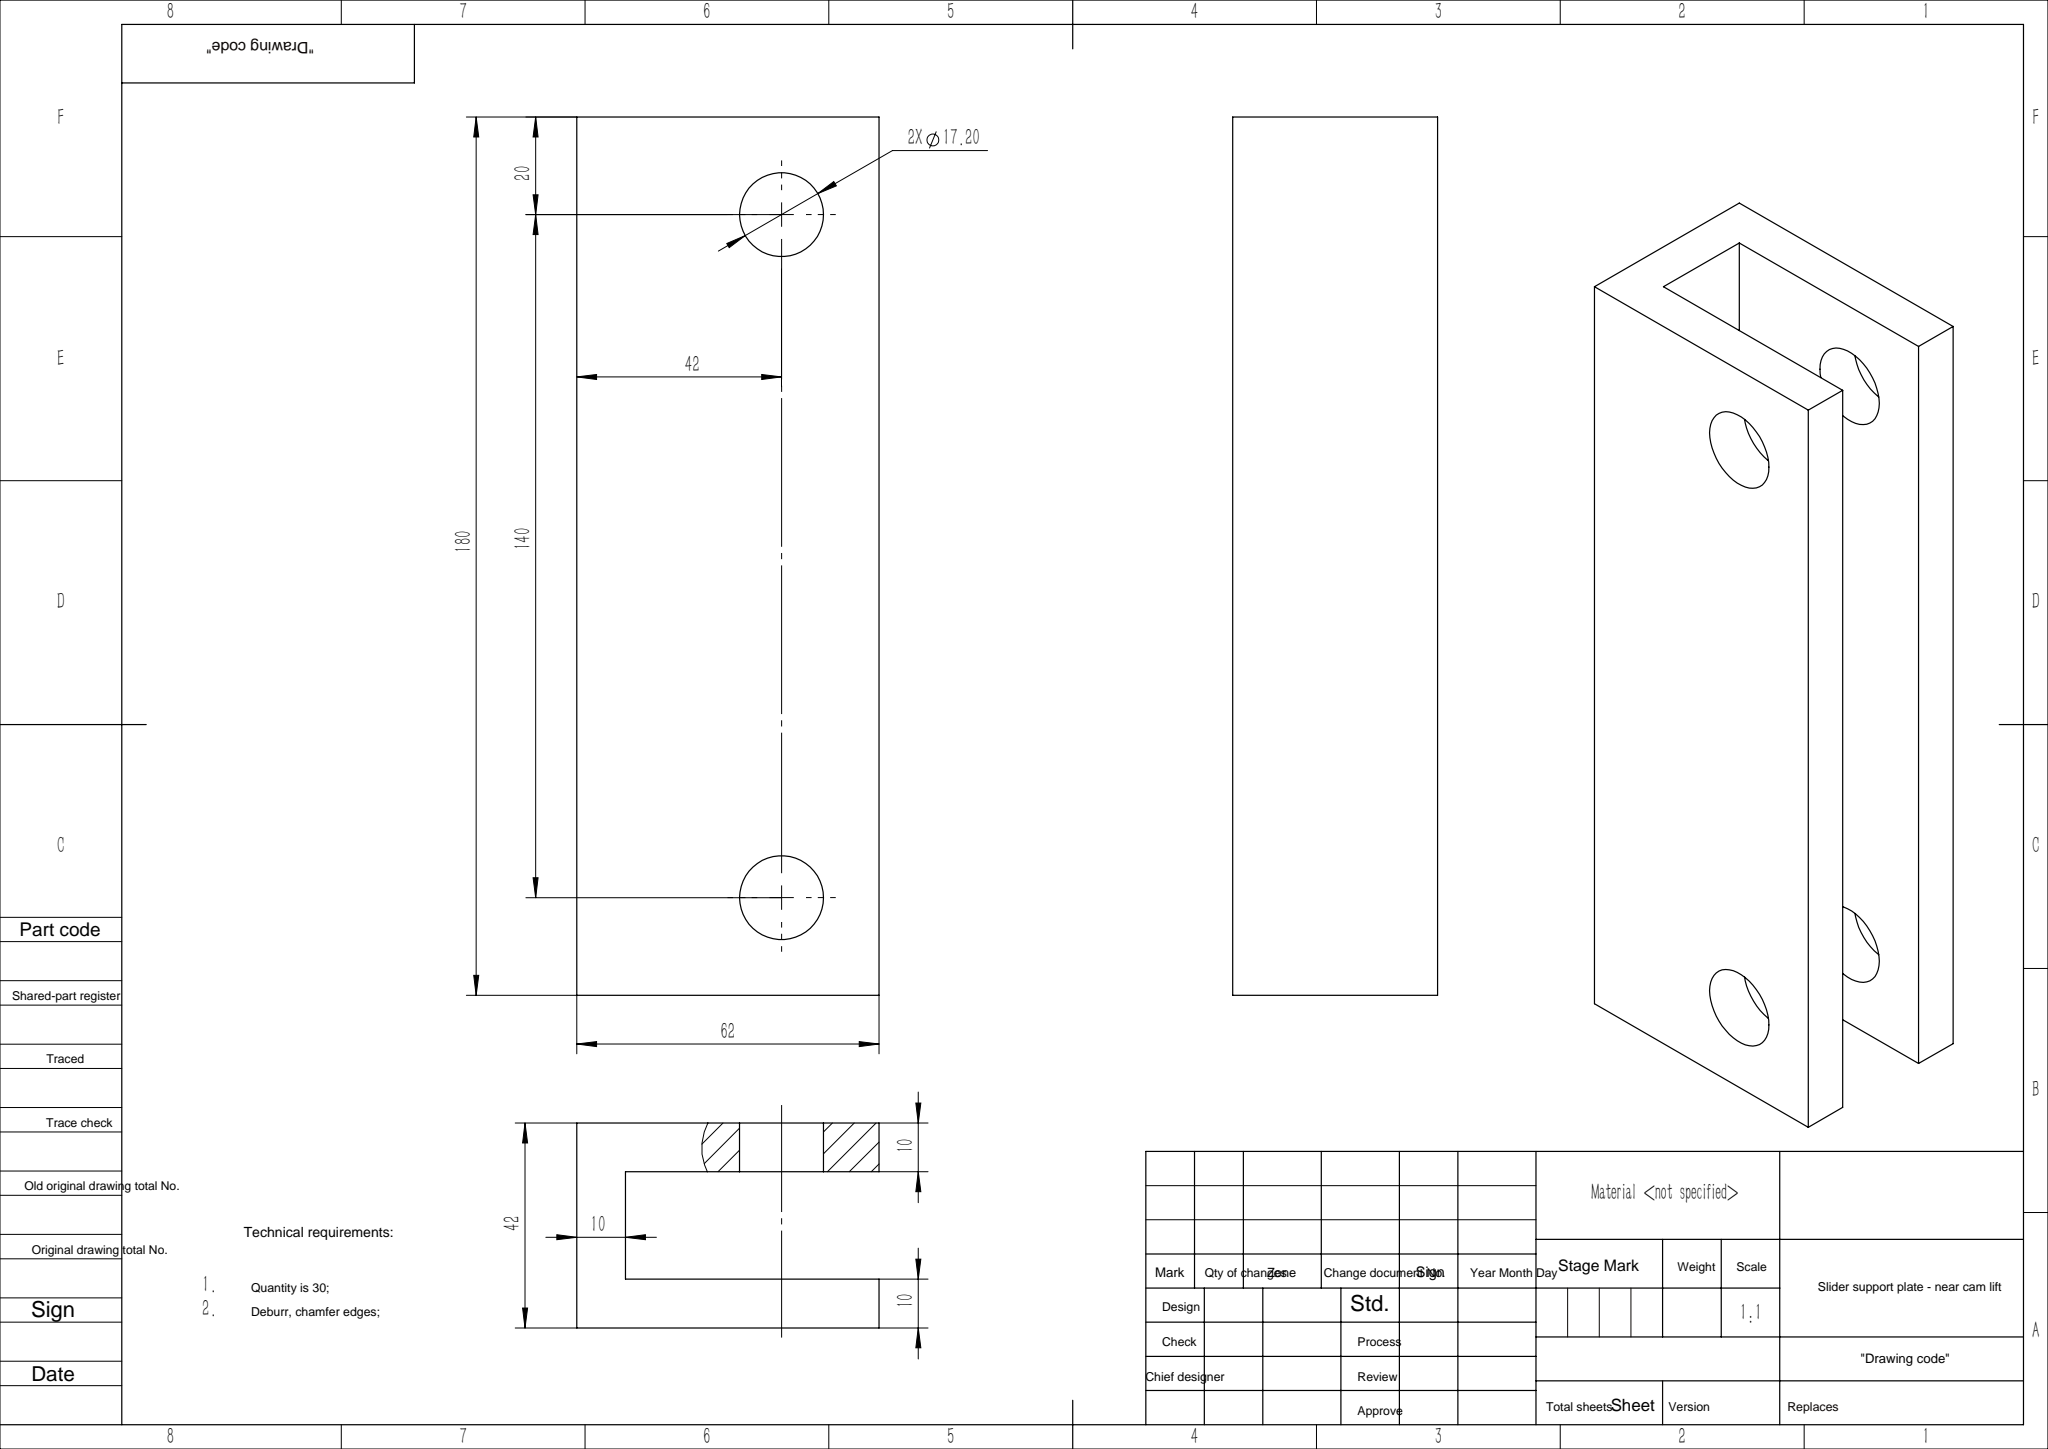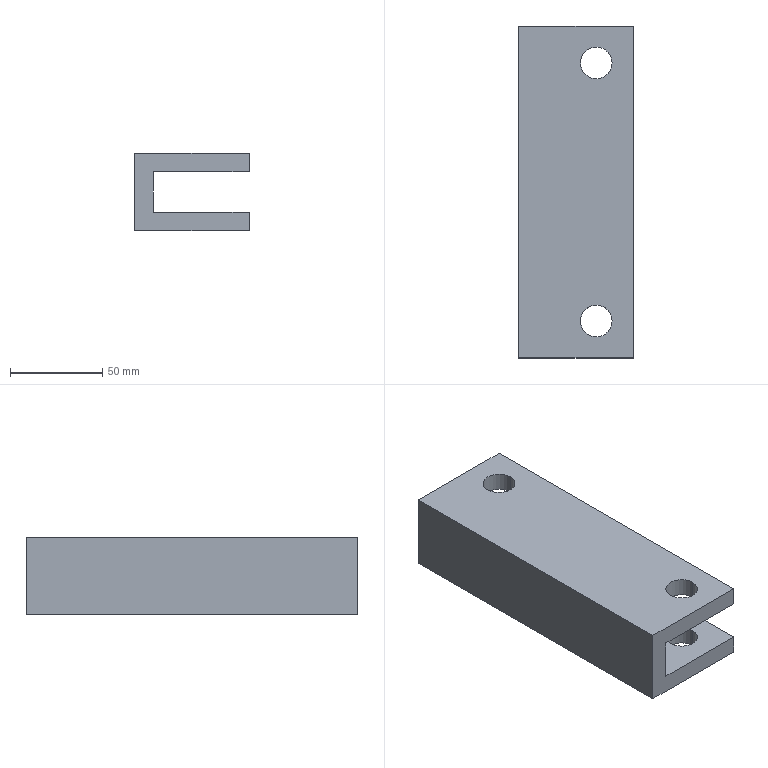Part | SolidWorks | features Extrusion 1, ICE 1 | 1 solid | 18 faces | box 62 x 180 x 42 mm | volume 253506 mm3 | plane 10 | cylinder 8 | commonest cylinder face diameters 17.2 x8
STEP:
#1=CARTESIAN_POINT('',(33.4,20.,11.));
#2=VERTEX_POINT('',#1);
#3=CARTESIAN_POINT('',(50.6,20.,11.));
#4=VERTEX_POINT('',#3);
#5=CARTESIAN_POINT('',(42.,20.,11.));
#6=DIRECTION('',(0.,0.,1.));
#7=DIRECTION('',(1.,0.,0.));
#8=AXIS2_PLACEMENT_3D('',#5,#6,#7);
#9=CIRCLE('',#8,8.6);
#10=EDGE_CURVE('',#2,#4,#9,.T.);
#11=ORIENTED_EDGE('',*,*,#10,.F.);
#12=CARTESIAN_POINT('',(33.4,20.,21.));
#13=VERTEX_POINT('',#12);
#14=CARTESIAN_POINT('',(33.4,20.,-21.));
#15=DIRECTION('',(0.,0.,1.));
#16=VECTOR('',#15,1000.);
#17=LINE('',#14,#16);
#18=EDGE_CURVE('',#2,#13,#17,.T.);
#19=ORIENTED_EDGE('',*,*,#18,.T.);
#20=CARTESIAN_POINT('',(50.6,20.,21.));
#21=VERTEX_POINT('',#20);
#22=CARTESIAN_POINT('',(42.,20.,21.));
#23=DIRECTION('',(0.,0.,1.));
#24=DIRECTION('',(1.,0.,0.));
#25=AXIS2_PLACEMENT_3D('',#22,#23,#24);
#26=CIRCLE('',#25,8.6);
#27=EDGE_CURVE('',#13,#21,#26,.T.);
#28=ORIENTED_EDGE('',*,*,#27,.T.);
#29=CARTESIAN_POINT('',(50.6,20.,-21.));
#30=DIRECTION('',(0.,0.,1.));
#31=VECTOR('',#30,1000.);
#32=LINE('',#29,#31);
#33=EDGE_CURVE('',#4,#21,#32,.T.);
#34=ORIENTED_EDGE('',*,*,#33,.F.);
#35=EDGE_LOOP('',(#11,#19,#28,#34));
#36=FACE_OUTER_BOUND('',#35,.T.);
#37=CARTESIAN_POINT('',(42.,20.,-21.));
#38=DIRECTION('',(0.,0.,1.));
#39=DIRECTION('',(1.,0.,0.));
#40=AXIS2_PLACEMENT_3D('',#37,#38,#39);
#41=CYLINDRICAL_SURFACE('',#40,8.6);
#42=ADVANCED_FACE('',(#36),#41,.F.);
#43=CARTESIAN_POINT('',(33.4,20.,-21.));
#44=VERTEX_POINT('',#43);
#45=CARTESIAN_POINT('',(50.6,20.,-21.));
#46=VERTEX_POINT('',#45);
#47=CARTESIAN_POINT('',(42.,20.,-21.));
#48=DIRECTION('',(0.,0.,1.));
#49=DIRECTION('',(1.,0.,0.));
#50=AXIS2_PLACEMENT_3D('',#47,#48,#49);
#51=CIRCLE('',#50,8.6);
#52=EDGE_CURVE('',#44,#46,#51,.T.);
#53=ORIENTED_EDGE('',*,*,#52,.F.);
#54=CARTESIAN_POINT('',(33.4,20.,-11.));
#55=VERTEX_POINT('',#54);
#56=CARTESIAN_POINT('',(33.4,20.,-21.));
#57=DIRECTION('',(0.,0.,1.));
#58=VECTOR('',#57,1000.);
#59=LINE('',#56,#58);
#60=EDGE_CURVE('',#44,#55,#59,.T.);
#61=ORIENTED_EDGE('',*,*,#60,.T.);
#62=CARTESIAN_POINT('',(50.6,20.,-11.));
#63=VERTEX_POINT('',#62);
#64=CARTESIAN_POINT('',(42.,20.,-11.));
#65=DIRECTION('',(0.,0.,-1.));
#66=DIRECTION('',(-1.,0.,0.));
#67=AXIS2_PLACEMENT_3D('',#64,#65,#66);
#68=CIRCLE('',#67,8.6);
#69=EDGE_CURVE('',#63,#55,#68,.T.);
#70=ORIENTED_EDGE('',*,*,#69,.F.);
#71=CARTESIAN_POINT('',(50.6,20.,-21.));
#72=DIRECTION('',(0.,0.,1.));
#73=VECTOR('',#72,1000.);
#74=LINE('',#71,#73);
#75=EDGE_CURVE('',#46,#63,#74,.T.);
#76=ORIENTED_EDGE('',*,*,#75,.F.);
#77=EDGE_LOOP('',(#53,#61,#70,#76));
#78=FACE_OUTER_BOUND('',#77,.T.);
#79=CARTESIAN_POINT('',(42.,20.,-21.));
#80=DIRECTION('',(0.,0.,1.));
#81=DIRECTION('',(1.,0.,0.));
#82=AXIS2_PLACEMENT_3D('',#79,#80,#81);
#83=CYLINDRICAL_SURFACE('',#82,8.6);
#84=ADVANCED_FACE('',(#78),#83,.F.);
#85=CARTESIAN_POINT('',(33.4,160.,11.));
#86=VERTEX_POINT('',#85);
#87=CARTESIAN_POINT('',(50.6,160.,11.));
#88=VERTEX_POINT('',#87);
#89=CARTESIAN_POINT('',(42.,160.,11.));
#90=DIRECTION('',(0.,0.,1.));
#91=DIRECTION('',(1.,0.,0.));
#92=AXIS2_PLACEMENT_3D('',#89,#90,#91);
#93=CIRCLE('',#92,8.6);
#94=EDGE_CURVE('',#86,#88,#93,.T.);
#95=ORIENTED_EDGE('',*,*,#94,.F.);
#96=CARTESIAN_POINT('',(33.4,160.,21.));
#97=VERTEX_POINT('',#96);
#98=CARTESIAN_POINT('',(33.4,160.,-21.));
#99=DIRECTION('',(0.,0.,1.));
#100=VECTOR('',#99,1000.);
#101=LINE('',#98,#100);
#102=EDGE_CURVE('',#86,#97,#101,.T.);
#103=ORIENTED_EDGE('',*,*,#102,.T.);
#104=CARTESIAN_POINT('',(50.6,160.,21.));
#105=VERTEX_POINT('',#104);
#106=CARTESIAN_POINT('',(42.,160.,21.));
#107=DIRECTION('',(0.,0.,1.));
#108=DIRECTION('',(1.,0.,0.));
#109=AXIS2_PLACEMENT_3D('',#106,#107,#108);
#110=CIRCLE('',#109,8.6);
#111=EDGE_CURVE('',#97,#105,#110,.T.);
#112=ORIENTED_EDGE('',*,*,#111,.T.);
#113=CARTESIAN_POINT('',(50.6,160.,-21.));
#114=DIRECTION('',(0.,0.,1.));
#115=VECTOR('',#114,1000.);
#116=LINE('',#113,#115);
#117=EDGE_CURVE('',#88,#105,#116,.T.);
#118=ORIENTED_EDGE('',*,*,#117,.F.);
#119=EDGE_LOOP('',(#95,#103,#112,#118));
#120=FACE_OUTER_BOUND('',#119,.T.);
#121=CARTESIAN_POINT('',(42.,160.,-21.));
#122=DIRECTION('',(0.,0.,1.));
#123=DIRECTION('',(1.,0.,0.));
#124=AXIS2_PLACEMENT_3D('',#121,#122,#123);
#125=CYLINDRICAL_SURFACE('',#124,8.6);
#126=ADVANCED_FACE('',(#120),#125,.F.);
#127=CARTESIAN_POINT('',(33.4,160.,-21.));
#128=VERTEX_POINT('',#127);
#129=CARTESIAN_POINT('',(50.6,160.,-21.));
#130=VERTEX_POINT('',#129);
#131=CARTESIAN_POINT('',(42.,160.,-21.));
#132=DIRECTION('',(0.,0.,1.));
#133=DIRECTION('',(1.,0.,0.));
#134=AXIS2_PLACEMENT_3D('',#131,#132,#133);
#135=CIRCLE('',#134,8.6);
#136=EDGE_CURVE('',#128,#130,#135,.T.);
#137=ORIENTED_EDGE('',*,*,#136,.F.);
#138=CARTESIAN_POINT('',(33.4,160.,-11.));
#139=VERTEX_POINT('',#138);
#140=CARTESIAN_POINT('',(33.4,160.,-21.));
#141=DIRECTION('',(0.,0.,1.));
#142=VECTOR('',#141,1000.);
#143=LINE('',#140,#142);
#144=EDGE_CURVE('',#128,#139,#143,.T.);
#145=ORIENTED_EDGE('',*,*,#144,.T.);
#146=CARTESIAN_POINT('',(50.6,160.,-11.));
#147=VERTEX_POINT('',#146);
#148=CARTESIAN_POINT('',(42.,160.,-11.));
#149=DIRECTION('',(0.,0.,-1.));
#150=DIRECTION('',(-1.,0.,0.));
#151=AXIS2_PLACEMENT_3D('',#148,#149,#150);
#152=CIRCLE('',#151,8.6);
#153=EDGE_CURVE('',#147,#139,#152,.T.);
#154=ORIENTED_EDGE('',*,*,#153,.F.);
#155=CARTESIAN_POINT('',(50.6,160.,-21.));
#156=DIRECTION('',(0.,0.,1.));
#157=VECTOR('',#156,1000.);
#158=LINE('',#155,#157);
#159=EDGE_CURVE('',#130,#147,#158,.T.);
#160=ORIENTED_EDGE('',*,*,#159,.F.);
#161=EDGE_LOOP('',(#137,#145,#154,#160));
#162=FACE_OUTER_BOUND('',#161,.T.);
#163=CARTESIAN_POINT('',(42.,160.,-21.));
#164=DIRECTION('',(0.,0.,1.));
#165=DIRECTION('',(1.,0.,0.));
#166=AXIS2_PLACEMENT_3D('',#163,#164,#165);
#167=CYLINDRICAL_SURFACE('',#166,8.6);
#168=ADVANCED_FACE('',(#162),#167,.F.);
#169=CARTESIAN_POINT('',(0.,0.,-21.));
#170=VERTEX_POINT('',#169);
#171=CARTESIAN_POINT('',(0.,0.,21.));
#172=VERTEX_POINT('',#171);
#173=CARTESIAN_POINT('',(0.,0.,-21.));
#174=DIRECTION('',(0.,0.,1.));
#175=VECTOR('',#174,1000.);
#176=LINE('',#173,#175);
#177=EDGE_CURVE('',#170,#172,#176,.T.);
#178=ORIENTED_EDGE('',*,*,#177,.T.);
#179=CARTESIAN_POINT('',(0.,180.,21.));
#180=VERTEX_POINT('',#179);
#181=CARTESIAN_POINT('',(0.,180.,21.));
#182=DIRECTION('',(0.,-1.,0.));
#183=VECTOR('',#182,1000.);
#184=LINE('',#181,#183);
#185=EDGE_CURVE('',#180,#172,#184,.T.);
#186=ORIENTED_EDGE('',*,*,#185,.F.);
#187=CARTESIAN_POINT('',(0.,180.,-21.));
#188=VERTEX_POINT('',#187);
#189=CARTESIAN_POINT('',(0.,180.,-21.));
#190=DIRECTION('',(0.,0.,1.));
#191=VECTOR('',#190,1000.);
#192=LINE('',#189,#191);
#193=EDGE_CURVE('',#188,#180,#192,.T.);
#194=ORIENTED_EDGE('',*,*,#193,.F.);
#195=CARTESIAN_POINT('',(0.,180.,-21.));
#196=DIRECTION('',(0.,-1.,0.));
#197=VECTOR('',#196,1000.);
#198=LINE('',#195,#197);
#199=EDGE_CURVE('',#188,#170,#198,.T.);
#200=ORIENTED_EDGE('',*,*,#199,.T.);
#201=EDGE_LOOP('',(#178,#186,#194,#200));
#202=FACE_OUTER_BOUND('',#201,.T.);
#203=CARTESIAN_POINT('',(0.,180.,-21.));
#204=DIRECTION('',(1.,0.,0.));
#205=DIRECTION('',(0.,0.,-1.));
#206=AXIS2_PLACEMENT_3D('',#203,#204,#205);
#207=PLANE('',#206);
#208=ADVANCED_FACE('',(#202),#207,.F.);
#209=CARTESIAN_POINT('',(42.,20.,21.));
#210=DIRECTION('',(0.,0.,1.));
#211=DIRECTION('',(1.,0.,0.));
#212=AXIS2_PLACEMENT_3D('',#209,#210,#211);
#213=CIRCLE('',#212,8.6);
#214=EDGE_CURVE('',#21,#13,#213,.T.);
#215=ORIENTED_EDGE('',*,*,#214,.F.);
#216=ORIENTED_EDGE('',*,*,#27,.F.);
#217=EDGE_LOOP('',(#215,#216));
#218=FACE_BOUND('',#217,.T.);
#219=CARTESIAN_POINT('',(42.,160.,21.));
#220=DIRECTION('',(0.,0.,1.));
#221=DIRECTION('',(1.,0.,0.));
#222=AXIS2_PLACEMENT_3D('',#219,#220,#221);
#223=CIRCLE('',#222,8.6);
#224=EDGE_CURVE('',#105,#97,#223,.T.);
#225=ORIENTED_EDGE('',*,*,#224,.F.);
#226=ORIENTED_EDGE('',*,*,#111,.F.);
#227=EDGE_LOOP('',(#225,#226));
#228=FACE_BOUND('',#227,.T.);
#229=CARTESIAN_POINT('',(62.,0.,21.));
#230=VERTEX_POINT('',#229);
#231=CARTESIAN_POINT('',(0.,0.,21.));
#232=DIRECTION('',(1.,0.,0.));
#233=VECTOR('',#232,1000.);
#234=LINE('',#231,#233);
#235=EDGE_CURVE('',#172,#230,#234,.T.);
#236=ORIENTED_EDGE('',*,*,#235,.T.);
#237=CARTESIAN_POINT('',(62.,180.,21.));
#238=VERTEX_POINT('',#237);
#239=CARTESIAN_POINT('',(62.,180.,21.));
#240=DIRECTION('',(0.,-1.,0.));
#241=VECTOR('',#240,1000.);
#242=LINE('',#239,#241);
#243=EDGE_CURVE('',#238,#230,#242,.T.);
#244=ORIENTED_EDGE('',*,*,#243,.F.);
#245=CARTESIAN_POINT('',(0.,180.,21.));
#246=DIRECTION('',(1.,0.,0.));
#247=VECTOR('',#246,1000.);
#248=LINE('',#245,#247);
#249=EDGE_CURVE('',#180,#238,#248,.T.);
#250=ORIENTED_EDGE('',*,*,#249,.F.);
#251=ORIENTED_EDGE('',*,*,#185,.T.);
#252=EDGE_LOOP('',(#236,#244,#250,#251));
#253=FACE_OUTER_BOUND('',#252,.T.);
#254=CARTESIAN_POINT('',(0.,180.,21.));
#255=DIRECTION('',(0.,0.,-1.));
#256=DIRECTION('',(-1.,0.,0.));
#257=AXIS2_PLACEMENT_3D('',#254,#255,#256);
#258=PLANE('',#257);
#259=ADVANCED_FACE('',(#218,#228,#253),#258,.F.);
#260=CARTESIAN_POINT('',(62.,0.,11.));
#261=VERTEX_POINT('',#260);
#262=CARTESIAN_POINT('',(62.,0.,11.));
#263=DIRECTION('',(0.,0.,-1.));
#264=VECTOR('',#263,1000.);
#265=LINE('',#262,#264);
#266=EDGE_CURVE('',#230,#261,#265,.T.);
#267=ORIENTED_EDGE('',*,*,#266,.T.);
#268=CARTESIAN_POINT('',(62.,180.,11.));
#269=VERTEX_POINT('',#268);
#270=CARTESIAN_POINT('',(62.,180.,11.));
#271=DIRECTION('',(0.,-1.,0.));
#272=VECTOR('',#271,1000.);
#273=LINE('',#270,#272);
#274=EDGE_CURVE('',#269,#261,#273,.T.);
#275=ORIENTED_EDGE('',*,*,#274,.F.);
#276=CARTESIAN_POINT('',(62.,180.,11.));
#277=DIRECTION('',(0.,0.,-1.));
#278=VECTOR('',#277,1000.);
#279=LINE('',#276,#278);
#280=EDGE_CURVE('',#238,#269,#279,.T.);
#281=ORIENTED_EDGE('',*,*,#280,.F.);
#282=ORIENTED_EDGE('',*,*,#243,.T.);
#283=EDGE_LOOP('',(#267,#275,#281,#282));
#284=FACE_OUTER_BOUND('',#283,.T.);
#285=CARTESIAN_POINT('',(62.,180.,11.));
#286=DIRECTION('',(-1.,0.,0.));
#287=DIRECTION('',(0.,0.,1.));
#288=AXIS2_PLACEMENT_3D('',#285,#286,#287);
#289=PLANE('',#288);
#290=ADVANCED_FACE('',(#284),#289,.F.);
#291=CARTESIAN_POINT('',(42.,20.,11.));
#292=DIRECTION('',(0.,0.,1.));
#293=DIRECTION('',(1.,0.,0.));
#294=AXIS2_PLACEMENT_3D('',#291,#292,#293);
#295=CIRCLE('',#294,8.6);
#296=EDGE_CURVE('',#4,#2,#295,.T.);
#297=ORIENTED_EDGE('',*,*,#296,.T.);
#298=ORIENTED_EDGE('',*,*,#10,.T.);
#299=EDGE_LOOP('',(#297,#298));
#300=FACE_BOUND('',#299,.T.);
#301=CARTESIAN_POINT('',(42.,160.,11.));
#302=DIRECTION('',(0.,0.,1.));
#303=DIRECTION('',(1.,0.,0.));
#304=AXIS2_PLACEMENT_3D('',#301,#302,#303);
#305=CIRCLE('',#304,8.6);
#306=EDGE_CURVE('',#88,#86,#305,.T.);
#307=ORIENTED_EDGE('',*,*,#306,.T.);
#308=ORIENTED_EDGE('',*,*,#94,.T.);
#309=EDGE_LOOP('',(#307,#308));
#310=FACE_BOUND('',#309,.T.);
#311=CARTESIAN_POINT('',(10.,0.,11.));
#312=VERTEX_POINT('',#311);
#313=CARTESIAN_POINT('',(10.,0.,11.));
#314=DIRECTION('',(-1.,0.,0.));
#315=VECTOR('',#314,1000.);
#316=LINE('',#313,#315);
#317=EDGE_CURVE('',#261,#312,#316,.T.);
#318=ORIENTED_EDGE('',*,*,#317,.T.);
#319=CARTESIAN_POINT('',(10.,180.,11.));
#320=VERTEX_POINT('',#319);
#321=CARTESIAN_POINT('',(10.,180.,11.));
#322=DIRECTION('',(0.,-1.,0.));
#323=VECTOR('',#322,1000.);
#324=LINE('',#321,#323);
#325=EDGE_CURVE('',#320,#312,#324,.T.);
#326=ORIENTED_EDGE('',*,*,#325,.F.);
#327=CARTESIAN_POINT('',(10.,180.,11.));
#328=DIRECTION('',(-1.,0.,0.));
#329=VECTOR('',#328,1000.);
#330=LINE('',#327,#329);
#331=EDGE_CURVE('',#269,#320,#330,.T.);
#332=ORIENTED_EDGE('',*,*,#331,.F.);
#333=ORIENTED_EDGE('',*,*,#274,.T.);
#334=EDGE_LOOP('',(#318,#326,#332,#333));
#335=FACE_OUTER_BOUND('',#334,.T.);
#336=CARTESIAN_POINT('',(10.,180.,11.));
#337=DIRECTION('',(0.,0.,1.));
#338=DIRECTION('',(1.,0.,0.));
#339=AXIS2_PLACEMENT_3D('',#336,#337,#338);
#340=PLANE('',#339);
#341=ADVANCED_FACE('',(#300,#310,#335),#340,.F.);
#342=CARTESIAN_POINT('',(10.,0.,-11.));
#343=VERTEX_POINT('',#342);
#344=CARTESIAN_POINT('',(10.,0.,-11.));
#345=DIRECTION('',(0.,0.,-1.));
#346=VECTOR('',#345,1000.);
#347=LINE('',#344,#346);
#348=EDGE_CURVE('',#312,#343,#347,.T.);
#349=ORIENTED_EDGE('',*,*,#348,.T.);
#350=CARTESIAN_POINT('',(10.,180.,-11.));
#351=VERTEX_POINT('',#350);
#352=CARTESIAN_POINT('',(10.,180.,-11.));
#353=DIRECTION('',(0.,-1.,0.));
#354=VECTOR('',#353,1000.);
#355=LINE('',#352,#354);
#356=EDGE_CURVE('',#351,#343,#355,.T.);
#357=ORIENTED_EDGE('',*,*,#356,.F.);
#358=CARTESIAN_POINT('',(10.,180.,-11.));
#359=DIRECTION('',(0.,0.,-1.));
#360=VECTOR('',#359,1000.);
#361=LINE('',#358,#360);
#362=EDGE_CURVE('',#320,#351,#361,.T.);
#363=ORIENTED_EDGE('',*,*,#362,.F.);
#364=ORIENTED_EDGE('',*,*,#325,.T.);
#365=EDGE_LOOP('',(#349,#357,#363,#364));
#366=FACE_OUTER_BOUND('',#365,.T.);
#367=CARTESIAN_POINT('',(10.,180.,-11.));
#368=DIRECTION('',(-1.,0.,0.));
#369=DIRECTION('',(0.,0.,1.));
#370=AXIS2_PLACEMENT_3D('',#367,#368,#369);
#371=PLANE('',#370);
#372=ADVANCED_FACE('',(#366),#371,.F.);
#373=ORIENTED_EDGE('',*,*,#69,.T.);
#374=CARTESIAN_POINT('',(42.,20.,-11.));
#375=DIRECTION('',(0.,0.,-1.));
#376=DIRECTION('',(-1.,0.,0.));
#377=AXIS2_PLACEMENT_3D('',#374,#375,#376);
#378=CIRCLE('',#377,8.6);
#379=EDGE_CURVE('',#55,#63,#378,.T.);
#380=ORIENTED_EDGE('',*,*,#379,.T.);
#381=EDGE_LOOP('',(#373,#380));
#382=FACE_BOUND('',#381,.T.);
#383=ORIENTED_EDGE('',*,*,#153,.T.);
#384=CARTESIAN_POINT('',(42.,160.,-11.));
#385=DIRECTION('',(0.,0.,-1.));
#386=DIRECTION('',(-1.,0.,0.));
#387=AXIS2_PLACEMENT_3D('',#384,#385,#386);
#388=CIRCLE('',#387,8.6);
#389=EDGE_CURVE('',#139,#147,#388,.T.);
#390=ORIENTED_EDGE('',*,*,#389,.T.);
#391=EDGE_LOOP('',(#383,#390));
#392=FACE_BOUND('',#391,.T.);
#393=CARTESIAN_POINT('',(62.,0.,-11.));
#394=VERTEX_POINT('',#393);
#395=CARTESIAN_POINT('',(62.,0.,-11.));
#396=DIRECTION('',(1.,0.,0.));
#397=VECTOR('',#396,1000.);
#398=LINE('',#395,#397);
#399=EDGE_CURVE('',#343,#394,#398,.T.);
#400=ORIENTED_EDGE('',*,*,#399,.T.);
#401=CARTESIAN_POINT('',(62.,180.,-11.));
#402=VERTEX_POINT('',#401);
#403=CARTESIAN_POINT('',(62.,180.,-11.));
#404=DIRECTION('',(0.,-1.,0.));
#405=VECTOR('',#404,1000.);
#406=LINE('',#403,#405);
#407=EDGE_CURVE('',#402,#394,#406,.T.);
#408=ORIENTED_EDGE('',*,*,#407,.F.);
#409=CARTESIAN_POINT('',(62.,180.,-11.));
#410=DIRECTION('',(1.,0.,0.));
#411=VECTOR('',#410,1000.);
#412=LINE('',#409,#411);
#413=EDGE_CURVE('',#351,#402,#412,.T.);
#414=ORIENTED_EDGE('',*,*,#413,.F.);
#415=ORIENTED_EDGE('',*,*,#356,.T.);
#416=EDGE_LOOP('',(#400,#408,#414,#415));
#417=FACE_OUTER_BOUND('',#416,.T.);
#418=CARTESIAN_POINT('',(62.,180.,-11.));
#419=DIRECTION('',(0.,0.,-1.));
#420=DIRECTION('',(-1.,0.,0.));
#421=AXIS2_PLACEMENT_3D('',#418,#419,#420);
#422=PLANE('',#421);
#423=ADVANCED_FACE('',(#382,#392,#417),#422,.F.);
#424=CARTESIAN_POINT('',(62.,0.,-21.));
#425=VERTEX_POINT('',#424);
#426=CARTESIAN_POINT('',(62.,0.,-21.));
#427=DIRECTION('',(0.,0.,-1.));
#428=VECTOR('',#427,1000.);
#429=LINE('',#426,#428);
#430=EDGE_CURVE('',#394,#425,#429,.T.);
#431=ORIENTED_EDGE('',*,*,#430,.T.);
#432=CARTESIAN_POINT('',(62.,180.,-21.));
#433=VERTEX_POINT('',#432);
#434=CARTESIAN_POINT('',(62.,180.,-21.));
#435=DIRECTION('',(0.,-1.,0.));
#436=VECTOR('',#435,1000.);
#437=LINE('',#434,#436);
#438=EDGE_CURVE('',#433,#425,#437,.T.);
#439=ORIENTED_EDGE('',*,*,#438,.F.);
#440=CARTESIAN_POINT('',(62.,180.,-21.));
#441=DIRECTION('',(0.,0.,-1.));
#442=VECTOR('',#441,1000.);
#443=LINE('',#440,#442);
#444=EDGE_CURVE('',#402,#433,#443,.T.);
#445=ORIENTED_EDGE('',*,*,#444,.F.);
#446=ORIENTED_EDGE('',*,*,#407,.T.);
#447=EDGE_LOOP('',(#431,#439,#445,#446));
#448=FACE_OUTER_BOUND('',#447,.T.);
#449=CARTESIAN_POINT('',(62.,180.,-21.));
#450=DIRECTION('',(-1.,0.,0.));
#451=DIRECTION('',(0.,0.,1.));
#452=AXIS2_PLACEMENT_3D('',#449,#450,#451);
#453=PLANE('',#452);
#454=ADVANCED_FACE('',(#448),#453,.F.);
#455=CARTESIAN_POINT('',(42.,20.,-21.));
#456=DIRECTION('',(0.,0.,1.));
#457=DIRECTION('',(1.,0.,0.));
#458=AXIS2_PLACEMENT_3D('',#455,#456,#457);
#459=CIRCLE('',#458,8.6);
#460=EDGE_CURVE('',#46,#44,#459,.T.);
#461=ORIENTED_EDGE('',*,*,#460,.T.);
#462=ORIENTED_EDGE('',*,*,#52,.T.);
#463=EDGE_LOOP('',(#461,#462));
#464=FACE_BOUND('',#463,.T.);
#465=CARTESIAN_POINT('',(42.,160.,-21.));
#466=DIRECTION('',(0.,0.,1.));
#467=DIRECTION('',(1.,0.,0.));
#468=AXIS2_PLACEMENT_3D('',#465,#466,#467);
#469=CIRCLE('',#468,8.6);
#470=EDGE_CURVE('',#130,#128,#469,.T.);
#471=ORIENTED_EDGE('',*,*,#470,.T.);
#472=ORIENTED_EDGE('',*,*,#136,.T.);
#473=EDGE_LOOP('',(#471,#472));
#474=FACE_BOUND('',#473,.T.);
#475=CARTESIAN_POINT('',(0.,0.,-21.));
#476=DIRECTION('',(-1.,0.,0.));
#477=VECTOR('',#476,1000.);
#478=LINE('',#475,#477);
#479=EDGE_CURVE('',#425,#170,#478,.T.);
#480=ORIENTED_EDGE('',*,*,#479,.T.);
#481=ORIENTED_EDGE('',*,*,#199,.F.);
#482=CARTESIAN_POINT('',(0.,180.,-21.));
#483=DIRECTION('',(-1.,0.,0.));
#484=VECTOR('',#483,1000.);
#485=LINE('',#482,#484);
#486=EDGE_CURVE('',#433,#188,#485,.T.);
#487=ORIENTED_EDGE('',*,*,#486,.F.);
#488=ORIENTED_EDGE('',*,*,#438,.T.);
#489=EDGE_LOOP('',(#480,#481,#487,#488));
#490=FACE_OUTER_BOUND('',#489,.T.);
#491=CARTESIAN_POINT('',(0.,180.,-21.));
#492=DIRECTION('',(0.,0.,1.));
#493=DIRECTION('',(1.,0.,0.));
#494=AXIS2_PLACEMENT_3D('',#491,#492,#493);
#495=PLANE('',#494);
#496=ADVANCED_FACE('',(#464,#474,#490),#495,.F.);
#497=ORIENTED_EDGE('',*,*,#193,.T.);
#498=ORIENTED_EDGE('',*,*,#249,.T.);
#499=ORIENTED_EDGE('',*,*,#280,.T.);
#500=ORIENTED_EDGE('',*,*,#331,.T.);
#501=ORIENTED_EDGE('',*,*,#362,.T.);
#502=ORIENTED_EDGE('',*,*,#413,.T.);
#503=ORIENTED_EDGE('',*,*,#444,.T.);
#504=ORIENTED_EDGE('',*,*,#486,.T.);
#505=EDGE_LOOP('',(#497,#498,#499,#500,#501,#502,#503,#504));
#506=FACE_OUTER_BOUND('',#505,.T.);
#507=CARTESIAN_POINT('',(0.,180.,0.));
#508=DIRECTION('',(0.,1.,0.));
#509=DIRECTION('',(0.,0.,1.));
#510=AXIS2_PLACEMENT_3D('',#507,#508,#509);
#511=PLANE('',#510);
#512=ADVANCED_FACE('',(#506),#511,.T.);
#513=ORIENTED_EDGE('',*,*,#177,.F.);
#514=ORIENTED_EDGE('',*,*,#479,.F.);
#515=ORIENTED_EDGE('',*,*,#430,.F.);
#516=ORIENTED_EDGE('',*,*,#399,.F.);
#517=ORIENTED_EDGE('',*,*,#348,.F.);
#518=ORIENTED_EDGE('',*,*,#317,.F.);
#519=ORIENTED_EDGE('',*,*,#266,.F.);
#520=ORIENTED_EDGE('',*,*,#235,.F.);
#521=EDGE_LOOP('',(#513,#514,#515,#516,#517,#518,#519,#520));
#522=FACE_OUTER_BOUND('',#521,.T.);
#523=CARTESIAN_POINT('',(0.,0.,0.));
#524=DIRECTION('',(0.,1.,0.));
#525=DIRECTION('',(0.,0.,1.));
#526=AXIS2_PLACEMENT_3D('',#523,#524,#525);
#527=PLANE('',#526);
#528=ADVANCED_FACE('',(#522),#527,.F.);
#529=ORIENTED_EDGE('',*,*,#144,.F.);
#530=ORIENTED_EDGE('',*,*,#470,.F.);
#531=ORIENTED_EDGE('',*,*,#159,.T.);
#532=ORIENTED_EDGE('',*,*,#389,.F.);
#533=EDGE_LOOP('',(#529,#530,#531,#532));
#534=FACE_OUTER_BOUND('',#533,.T.);
#535=CARTESIAN_POINT('',(42.,160.,-21.));
#536=DIRECTION('',(0.,0.,1.));
#537=DIRECTION('',(1.,0.,0.));
#538=AXIS2_PLACEMENT_3D('',#535,#536,#537);
#539=CYLINDRICAL_SURFACE('',#538,8.6);
#540=ADVANCED_FACE('',(#534),#539,.F.);
#541=ORIENTED_EDGE('',*,*,#102,.F.);
#542=ORIENTED_EDGE('',*,*,#306,.F.);
#543=ORIENTED_EDGE('',*,*,#117,.T.);
#544=ORIENTED_EDGE('',*,*,#224,.T.);
#545=EDGE_LOOP('',(#541,#542,#543,#544));
#546=FACE_OUTER_BOUND('',#545,.T.);
#547=CARTESIAN_POINT('',(42.,160.,-21.));
#548=DIRECTION('',(0.,0.,1.));
#549=DIRECTION('',(1.,0.,0.));
#550=AXIS2_PLACEMENT_3D('',#547,#548,#549);
#551=CYLINDRICAL_SURFACE('',#550,8.6);
#552=ADVANCED_FACE('',(#546),#551,.F.);
#553=ORIENTED_EDGE('',*,*,#60,.F.);
#554=ORIENTED_EDGE('',*,*,#460,.F.);
#555=ORIENTED_EDGE('',*,*,#75,.T.);
#556=ORIENTED_EDGE('',*,*,#379,.F.);
#557=EDGE_LOOP('',(#553,#554,#555,#556));
#558=FACE_OUTER_BOUND('',#557,.T.);
#559=CARTESIAN_POINT('',(42.,20.,-21.));
#560=DIRECTION('',(0.,0.,1.));
#561=DIRECTION('',(1.,0.,0.));
#562=AXIS2_PLACEMENT_3D('',#559,#560,#561);
#563=CYLINDRICAL_SURFACE('',#562,8.6);
#564=ADVANCED_FACE('',(#558),#563,.F.);
#565=ORIENTED_EDGE('',*,*,#18,.F.);
#566=ORIENTED_EDGE('',*,*,#296,.F.);
#567=ORIENTED_EDGE('',*,*,#33,.T.);
#568=ORIENTED_EDGE('',*,*,#214,.T.);
#569=EDGE_LOOP('',(#565,#566,#567,#568));
#570=FACE_OUTER_BOUND('',#569,.T.);
#571=CARTESIAN_POINT('',(42.,20.,-21.));
#572=DIRECTION('',(0.,0.,1.));
#573=DIRECTION('',(1.,0.,0.));
#574=AXIS2_PLACEMENT_3D('',#571,#572,#573);
#575=CYLINDRICAL_SURFACE('',#574,8.6);
#576=ADVANCED_FACE('',(#570),#575,.F.);
#577=CLOSED_SHELL('',(#42,#84,#126,#168,#208,#259,#290,#341,#372,#423,#454,#496,#512,#528,#540,#552,#564,#576));
#578=MANIFOLD_SOLID_BREP('',#577);
#579=CARTESIAN_POINT('',(0.,0.,0.));
#580=DIRECTION('',(0.,0.,1.));
#581=DIRECTION('',(1.,0.,0.));
#582=AXIS2_PLACEMENT_3D('',#579,#580,#581);
#583=(LENGTH_UNIT()NAMED_UNIT(*)SI_UNIT(.MILLI.,.METRE.));
#584=UNCERTAINTY_MEASURE_WITH_UNIT(LENGTH_MEASURE(0.00001),#583,'','');
#585=(NAMED_UNIT(*)PLANE_ANGLE_UNIT()SI_UNIT($,.RADIAN.));
#586=(NAMED_UNIT(*)SI_UNIT($,.STERADIAN.)SOLID_ANGLE_UNIT());
#587=(GEOMETRIC_REPRESENTATION_CONTEXT(3)GLOBAL_UNCERTAINTY_ASSIGNED_CONTEXT((#584))GLOBAL_UNIT_ASSIGNED_CONTEXT((#583,#585,#586))REPRESENTATION_CONTEXT('',''));
#588=ADVANCED_BREP_SHAPE_REPRESENTATION('',(#578,#582),#587);